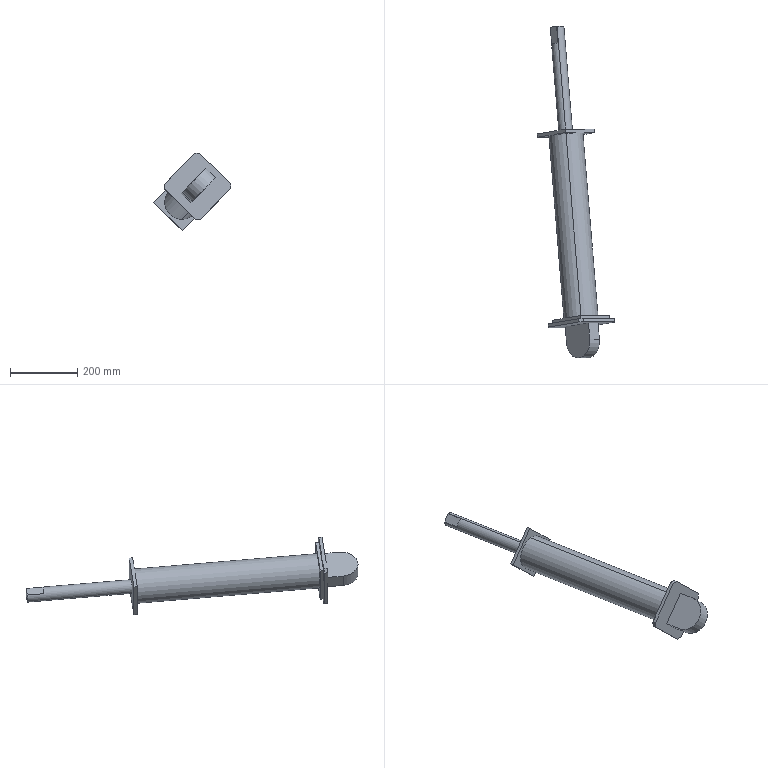Part | SolidWorks | features BaseBody 1 | 1 solid | 35 faces | box 230.771 x 990.893 x 231.743 mm | volume 5798117 mm3 | plane 30 | cylinder 5 | commonest cylinder face diameters 40.723 x2 102.404 x2 100 x1
STEP:
#1=CARTESIAN_POINT('',(-1330.685,834.679,-2427.636));
#2=VERTEX_POINT('',#1);
#3=CARTESIAN_POINT('',(-1330.685,843.27,-2325.593));
#4=VERTEX_POINT('',#3);
#5=CARTESIAN_POINT('',(-1330.685,838.974,-2376.614));
#6=DIRECTION('',(0.08182,-0.9931,0.08361));
#7=DIRECTION('',(0.,-0.08389,-0.9965));
#8=AXIS2_PLACEMENT_3D('',#5,#6,#7);
#9=CIRCLE('',#8,51.202);
#10=EDGE_CURVE('',#2,#4,#9,.T.);
#11=ORIENTED_EDGE('',*,*,#10,.T.);
#12=CARTESIAN_POINT('',(-1285.682,297.046,-2279.609));
#13=VERTEX_POINT('',#12);
#14=CARTESIAN_POINT('',(-1330.685,843.27,-2325.593));
#15=DIRECTION('',(0.08182,-0.9931,0.08361));
#16=VECTOR('',#15,1000.);
#17=LINE('',#14,#16);
#18=EDGE_CURVE('',#4,#13,#17,.T.);
#19=ORIENTED_EDGE('',*,*,#18,.T.);
#20=CARTESIAN_POINT('',(-1285.682,288.456,-2381.652));
#21=VERTEX_POINT('',#20);
#22=CARTESIAN_POINT('',(-1285.682,292.751,-2330.631));
#23=DIRECTION('',(-0.08182,0.9931,-0.08361));
#24=DIRECTION('',(0.,-0.08389,-0.9965));
#25=AXIS2_PLACEMENT_3D('',#22,#23,#24);
#26=CIRCLE('',#25,51.202);
#27=EDGE_CURVE('',#13,#21,#26,.T.);
#28=ORIENTED_EDGE('',*,*,#27,.T.);
#29=CARTESIAN_POINT('',(-1330.685,834.679,-2427.636));
#30=DIRECTION('',(0.08182,-0.9931,0.08361));
#31=VECTOR('',#30,1000.);
#32=LINE('',#29,#31);
#33=EDGE_CURVE('',#2,#21,#32,.T.);
#34=ORIENTED_EDGE('',*,*,#33,.F.);
#35=EDGE_LOOP('',(#11,#19,#28,#34));
#36=FACE_OUTER_BOUND('',#35,.T.);
#37=CARTESIAN_POINT('',(-1330.685,838.974,-2376.614));
#38=DIRECTION('',(0.08182,-0.9931,0.08361));
#39=DIRECTION('',(0.,-0.08389,-0.9965));
#40=AXIS2_PLACEMENT_3D('',#37,#38,#39);
#41=CYLINDRICAL_SURFACE('',#40,51.202);
#42=ADVANCED_FACE('',(#36),#41,.T.);
#43=CARTESIAN_POINT('',(-1336.993,1163.354,-2404.505));
#44=VERTEX_POINT('',#43);
#45=CARTESIAN_POINT('',(-1357.278,1163.451,-2383.497));
#46=VERTEX_POINT('',#45);
#47=CARTESIAN_POINT('',(-1357.278,1161.743,-2403.786));
#48=DIRECTION('',(0.08182,-0.9931,0.08361));
#49=DIRECTION('',(0.,-0.08389,-0.9965));
#50=AXIS2_PLACEMENT_3D('',#47,#48,#49);
#51=CIRCLE('',#50,20.361);
#52=EDGE_CURVE('',#44,#46,#51,.T.);
#53=ORIENTED_EDGE('',*,*,#52,.T.);
#54=CARTESIAN_POINT('',(-1331.503,850.614,-2357.161));
#55=VERTEX_POINT('',#54);
#56=CARTESIAN_POINT('',(-1357.278,1163.451,-2383.497));
#57=DIRECTION('',(0.08182,-0.9931,0.08361));
#58=VECTOR('',#57,1000.);
#59=LINE('',#56,#58);
#60=EDGE_CURVE('',#46,#55,#59,.T.);
#61=ORIENTED_EDGE('',*,*,#60,.T.);
#62=CARTESIAN_POINT('',(-1331.503,847.198,-2397.74));
#63=VERTEX_POINT('',#62);
#64=CARTESIAN_POINT('',(-1331.503,848.906,-2377.45));
#65=DIRECTION('',(0.08182,-0.9931,0.08361));
#66=DIRECTION('',(0.,-0.08389,-0.9965));
#67=AXIS2_PLACEMENT_3D('',#64,#65,#66);
#68=CIRCLE('',#67,20.361);
#69=EDGE_CURVE('',#63,#55,#68,.T.);
#70=ORIENTED_EDGE('',*,*,#69,.F.);
#71=CARTESIAN_POINT('',(-1357.278,1160.035,-2424.076));
#72=VERTEX_POINT('',#71);
#73=CARTESIAN_POINT('',(-1357.278,1160.035,-2424.076));
#74=DIRECTION('',(0.08182,-0.9931,0.08361));
#75=VECTOR('',#74,1000.);
#76=LINE('',#73,#75);
#77=EDGE_CURVE('',#72,#63,#76,.T.);
#78=ORIENTED_EDGE('',*,*,#77,.F.);
#79=CARTESIAN_POINT('',(-1356.122,1160.132,-2424.051));
#80=VERTEX_POINT('',#79);
#81=CARTESIAN_POINT('',(-1357.278,1161.743,-2403.786));
#82=DIRECTION('',(0.08182,-0.9931,0.08361));
#83=DIRECTION('',(0.,-0.08389,-0.9965));
#84=AXIS2_PLACEMENT_3D('',#81,#82,#83);
#85=CIRCLE('',#84,20.361);
#86=EDGE_CURVE('',#72,#80,#85,.T.);
#87=ORIENTED_EDGE('',*,*,#86,.T.);
#88=CARTESIAN_POINT('',(-1352.031,1110.475,-2419.871));
#89=VERTEX_POINT('',#88);
#90=CARTESIAN_POINT('',(-1356.122,1160.132,-2424.051));
#91=DIRECTION('',(0.08182,-0.9931,0.08361));
#92=VECTOR('',#91,1000.);
#93=LINE('',#90,#92);
#94=EDGE_CURVE('',#80,#89,#93,.T.);
#95=ORIENTED_EDGE('',*,*,#94,.T.);
#96=CARTESIAN_POINT('',(-1332.902,1113.697,-2400.325));
#97=VERTEX_POINT('',#96);
#98=CARTESIAN_POINT('',(-1353.186,1112.086,-2399.606));
#99=DIRECTION('',(0.08182,-0.9931,0.08361));
#100=DIRECTION('',(0.,-0.08389,-0.9965));
#101=AXIS2_PLACEMENT_3D('',#98,#99,#100);
#102=CIRCLE('',#101,20.361);
#103=EDGE_CURVE('',#89,#97,#102,.T.);
#104=ORIENTED_EDGE('',*,*,#103,.T.);
#105=CARTESIAN_POINT('',(-1336.993,1163.354,-2404.505));
#106=DIRECTION('',(-0.08182,0.9931,-0.08361));
#107=VECTOR('',#106,1000.);
#108=LINE('',#105,#107);
#109=EDGE_CURVE('',#97,#44,#108,.T.);
#110=ORIENTED_EDGE('',*,*,#109,.T.);
#111=EDGE_LOOP('',(#53,#61,#70,#78,#87,#95,#104,#110));
#112=FACE_OUTER_BOUND('',#111,.T.);
#113=CARTESIAN_POINT('',(-1357.278,1161.743,-2403.786));
#114=DIRECTION('',(0.08182,-0.9931,0.08361));
#115=DIRECTION('',(0.,-0.08389,-0.9965));
#116=AXIS2_PLACEMENT_3D('',#113,#114,#115);
#117=CYLINDRICAL_SURFACE('',#116,20.361);
#118=ADVANCED_FACE('',(#112),#117,.T.);
#119=ORIENTED_EDGE('',*,*,#18,.F.);
#120=CARTESIAN_POINT('',(-1330.685,838.974,-2376.614));
#121=DIRECTION('',(0.08182,-0.9931,0.08361));
#122=DIRECTION('',(0.,-0.08389,-0.9965));
#123=AXIS2_PLACEMENT_3D('',#120,#121,#122);
#124=CIRCLE('',#123,51.202);
#125=EDGE_CURVE('',#4,#2,#124,.T.);
#126=ORIENTED_EDGE('',*,*,#125,.T.);
#127=ORIENTED_EDGE('',*,*,#33,.T.);
#128=CARTESIAN_POINT('',(-1285.682,292.751,-2330.631));
#129=DIRECTION('',(-0.08182,0.9931,-0.08361));
#130=DIRECTION('',(0.,-0.08389,-0.9965));
#131=AXIS2_PLACEMENT_3D('',#128,#129,#130);
#132=CIRCLE('',#131,51.202);
#133=EDGE_CURVE('',#21,#13,#132,.T.);
#134=ORIENTED_EDGE('',*,*,#133,.T.);
#135=EDGE_LOOP('',(#119,#126,#127,#134));
#136=FACE_OUTER_BOUND('',#135,.T.);
#137=CARTESIAN_POINT('',(-1330.685,838.974,-2376.614));
#138=DIRECTION('',(0.08182,-0.9931,0.08361));
#139=DIRECTION('',(0.,-0.08389,-0.9965));
#140=AXIS2_PLACEMENT_3D('',#137,#138,#139);
#141=CYLINDRICAL_SURFACE('',#140,51.202);
#142=ADVANCED_FACE('',(#136),#141,.T.);
#143=ORIENTED_EDGE('',*,*,#10,.F.);
#144=ORIENTED_EDGE('',*,*,#125,.F.);
#145=EDGE_LOOP('',(#143,#144));
#146=FACE_BOUND('',#145,.T.);
#147=CARTESIAN_POINT('',(-1329.482,831.955,-2461.168));
#148=VERTEX_POINT('',#147);
#149=CARTESIAN_POINT('',(-1415.245,831.955,-2377.234));
#150=VERTEX_POINT('',#149);
#151=CARTESIAN_POINT('',(-1329.482,831.955,-2461.168));
#152=DIRECTION('',(-0.7147,0.,0.6994));
#153=VECTOR('',#152,1000.);
#154=LINE('',#151,#153);
#155=EDGE_CURVE('',#148,#150,#154,.T.);
#156=ORIENTED_EDGE('',*,*,#155,.F.);
#157=CARTESIAN_POINT('',(-1246.125,845.993,-2375.994));
#158=VERTEX_POINT('',#157);
#159=CARTESIAN_POINT('',(-1246.125,845.993,-2375.994));
#160=DIRECTION('',(-0.6946,-0.117,-0.7098));
#161=VECTOR('',#160,1000.);
#162=LINE('',#159,#161);
#163=EDGE_CURVE('',#158,#148,#162,.T.);
#164=ORIENTED_EDGE('',*,*,#163,.F.);
#165=CARTESIAN_POINT('',(-1331.888,845.993,-2292.061));
#166=VERTEX_POINT('',#165);
#167=CARTESIAN_POINT('',(-1331.888,845.993,-2292.061));
#168=DIRECTION('',(0.7147,0.,-0.6994));
#169=VECTOR('',#168,1000.);
#170=LINE('',#167,#169);
#171=EDGE_CURVE('',#166,#158,#170,.T.);
#172=ORIENTED_EDGE('',*,*,#171,.F.);
#173=CARTESIAN_POINT('',(-1415.245,831.955,-2377.234));
#174=DIRECTION('',(0.6946,0.117,0.7098));
#175=VECTOR('',#174,1000.);
#176=LINE('',#173,#175);
#177=EDGE_CURVE('',#150,#166,#176,.T.);
#178=ORIENTED_EDGE('',*,*,#177,.F.);
#179=EDGE_LOOP('',(#156,#164,#172,#178));
#180=FACE_OUTER_BOUND('',#179,.T.);
#181=CARTESIAN_POINT('',(-1330.685,838.974,-2376.614));
#182=DIRECTION('',(-0.08182,0.9931,-0.08361));
#183=DIRECTION('',(0.,0.08389,0.9965));
#184=AXIS2_PLACEMENT_3D('',#181,#182,#183);
#185=PLANE('',#184);
#186=ADVANCED_FACE('',(#146,#180),#185,.F.);
#187=ORIENTED_EDGE('',*,*,#133,.F.);
#188=ORIENTED_EDGE('',*,*,#27,.F.);
#189=EDGE_LOOP('',(#187,#188));
#190=FACE_BOUND('',#189,.T.);
#191=CARTESIAN_POINT('',(-1201.122,299.77,-2330.01));
#192=VERTEX_POINT('',#191);
#193=CARTESIAN_POINT('',(-1284.479,285.732,-2415.184));
#194=VERTEX_POINT('',#193);
#195=CARTESIAN_POINT('',(-1201.122,299.77,-2330.01));
#196=DIRECTION('',(-0.6946,-0.117,-0.7098));
#197=VECTOR('',#196,1000.);
#198=LINE('',#195,#197);
#199=EDGE_CURVE('',#192,#194,#198,.T.);
#200=ORIENTED_EDGE('',*,*,#199,.T.);
#201=CARTESIAN_POINT('',(-1370.242,285.732,-2331.251));
#202=VERTEX_POINT('',#201);
#203=CARTESIAN_POINT('',(-1284.479,285.732,-2415.184));
#204=DIRECTION('',(-0.7147,0.,0.6994));
#205=VECTOR('',#204,1000.);
#206=LINE('',#203,#205);
#207=EDGE_CURVE('',#194,#202,#206,.T.);
#208=ORIENTED_EDGE('',*,*,#207,.T.);
#209=CARTESIAN_POINT('',(-1286.885,299.77,-2246.077));
#210=VERTEX_POINT('',#209);
#211=CARTESIAN_POINT('',(-1370.242,285.732,-2331.251));
#212=DIRECTION('',(0.6946,0.117,0.7098));
#213=VECTOR('',#212,1000.);
#214=LINE('',#211,#213);
#215=EDGE_CURVE('',#202,#210,#214,.T.);
#216=ORIENTED_EDGE('',*,*,#215,.T.);
#217=CARTESIAN_POINT('',(-1286.885,299.77,-2246.077));
#218=DIRECTION('',(0.7147,0.,-0.6994));
#219=VECTOR('',#218,1000.);
#220=LINE('',#217,#219);
#221=EDGE_CURVE('',#210,#192,#220,.T.);
#222=ORIENTED_EDGE('',*,*,#221,.T.);
#223=EDGE_LOOP('',(#200,#208,#216,#222));
#224=FACE_OUTER_BOUND('',#223,.T.);
#225=CARTESIAN_POINT('',(-1285.682,292.751,-2330.631));
#226=DIRECTION('',(-0.08182,0.9931,-0.08361));
#227=DIRECTION('',(0.,0.08389,0.9965));
#228=AXIS2_PLACEMENT_3D('',#225,#226,#227);
#229=PLANE('',#228);
#230=ADVANCED_FACE('',(#190,#224),#229,.T.);
#231=CARTESIAN_POINT('',(-1332.706,855.925,-2292.897));
#232=VERTEX_POINT('',#231);
#233=CARTESIAN_POINT('',(-1332.706,855.925,-2292.897));
#234=DIRECTION('',(0.08182,-0.9931,0.08361));
#235=VECTOR('',#234,1000.);
#236=LINE('',#233,#235);
#237=EDGE_CURVE('',#232,#166,#236,.T.);
#238=ORIENTED_EDGE('',*,*,#237,.F.);
#239=CARTESIAN_POINT('',(-1416.063,841.887,-2378.07));
#240=VERTEX_POINT('',#239);
#241=CARTESIAN_POINT('',(-1416.063,841.887,-2378.07));
#242=DIRECTION('',(0.6946,0.117,0.7098));
#243=VECTOR('',#242,1000.);
#244=LINE('',#241,#243);
#245=EDGE_CURVE('',#240,#232,#244,.T.);
#246=ORIENTED_EDGE('',*,*,#245,.F.);
#247=CARTESIAN_POINT('',(-1415.245,831.955,-2377.234));
#248=DIRECTION('',(-0.08182,0.9931,-0.08361));
#249=VECTOR('',#248,1000.);
#250=LINE('',#247,#249);
#251=EDGE_CURVE('',#150,#240,#250,.T.);
#252=ORIENTED_EDGE('',*,*,#251,.F.);
#253=ORIENTED_EDGE('',*,*,#177,.T.);
#254=EDGE_LOOP('',(#238,#246,#252,#253));
#255=FACE_OUTER_BOUND('',#254,.T.);
#256=CARTESIAN_POINT('',(-1416.063,841.887,-2378.07));
#257=DIRECTION('',(0.7147,0.,-0.6994));
#258=DIRECTION('',(-0.6994,0.,-0.7147));
#259=AXIS2_PLACEMENT_3D('',#256,#257,#258);
#260=PLANE('',#259);
#261=ADVANCED_FACE('',(#255),#260,.F.);
#262=ORIENTED_EDGE('',*,*,#251,.T.);
#263=CARTESIAN_POINT('',(-1330.3,841.887,-2462.004));
#264=VERTEX_POINT('',#263);
#265=CARTESIAN_POINT('',(-1416.063,841.887,-2378.07));
#266=DIRECTION('',(-0.7147,0.,0.6994));
#267=VECTOR('',#266,1000.);
#268=LINE('',#265,#267);
#269=EDGE_CURVE('',#264,#240,#268,.T.);
#270=ORIENTED_EDGE('',*,*,#269,.F.);
#271=CARTESIAN_POINT('',(-1330.3,841.887,-2462.004));
#272=DIRECTION('',(-0.08182,0.9931,-0.08361));
#273=VECTOR('',#272,1000.);
#274=LINE('',#271,#273);
#275=EDGE_CURVE('',#148,#264,#274,.T.);
#276=ORIENTED_EDGE('',*,*,#275,.F.);
#277=ORIENTED_EDGE('',*,*,#155,.T.);
#278=EDGE_LOOP('',(#262,#270,#276,#277));
#279=FACE_OUTER_BOUND('',#278,.T.);
#280=CARTESIAN_POINT('',(-1416.063,841.887,-2378.07));
#281=DIRECTION('',(0.6946,0.117,0.7098));
#282=DIRECTION('',(0.7147,0.,-0.6994));
#283=AXIS2_PLACEMENT_3D('',#280,#281,#282);
#284=PLANE('',#283);
#285=ADVANCED_FACE('',(#279),#284,.F.);
#286=ORIENTED_EDGE('',*,*,#275,.T.);
#287=CARTESIAN_POINT('',(-1246.943,855.925,-2376.83));
#288=VERTEX_POINT('',#287);
#289=CARTESIAN_POINT('',(-1246.943,855.925,-2376.83));
#290=DIRECTION('',(-0.6946,-0.117,-0.7098));
#291=VECTOR('',#290,1000.);
#292=LINE('',#289,#291);
#293=EDGE_CURVE('',#288,#264,#292,.T.);
#294=ORIENTED_EDGE('',*,*,#293,.F.);
#295=CARTESIAN_POINT('',(-1246.125,845.993,-2375.994));
#296=DIRECTION('',(-0.08182,0.9931,-0.08361));
#297=VECTOR('',#296,1000.);
#298=LINE('',#295,#297);
#299=EDGE_CURVE('',#158,#288,#298,.T.);
#300=ORIENTED_EDGE('',*,*,#299,.F.);
#301=ORIENTED_EDGE('',*,*,#163,.T.);
#302=EDGE_LOOP('',(#286,#294,#300,#301));
#303=FACE_OUTER_BOUND('',#302,.T.);
#304=CARTESIAN_POINT('',(-1330.3,841.887,-2462.004));
#305=DIRECTION('',(-0.7147,0.,0.6994));
#306=DIRECTION('',(0.6994,0.,0.7147));
#307=AXIS2_PLACEMENT_3D('',#304,#305,#306);
#308=PLANE('',#307);
#309=ADVANCED_FACE('',(#303),#308,.F.);
#310=ORIENTED_EDGE('',*,*,#299,.T.);
#311=CARTESIAN_POINT('',(-1332.706,855.925,-2292.897));
#312=DIRECTION('',(0.7147,0.,-0.6994));
#313=VECTOR('',#312,1000.);
#314=LINE('',#311,#313);
#315=EDGE_CURVE('',#232,#288,#314,.T.);
#316=ORIENTED_EDGE('',*,*,#315,.F.);
#317=ORIENTED_EDGE('',*,*,#237,.T.);
#318=ORIENTED_EDGE('',*,*,#171,.T.);
#319=EDGE_LOOP('',(#310,#316,#317,#318));
#320=FACE_OUTER_BOUND('',#319,.T.);
#321=CARTESIAN_POINT('',(-1332.706,855.925,-2292.897));
#322=DIRECTION('',(-0.6946,-0.117,-0.7098));
#323=DIRECTION('',(-0.7147,0.,0.6994));
#324=AXIS2_PLACEMENT_3D('',#321,#322,#323);
#325=PLANE('',#324);
#326=ADVANCED_FACE('',(#320),#325,.F.);
#327=CARTESIAN_POINT('',(-1369.424,275.8,-2330.415));
#328=VERTEX_POINT('',#327);
#329=CARTESIAN_POINT('',(-1370.242,285.732,-2331.251));
#330=DIRECTION('',(0.08182,-0.9931,0.08361));
#331=VECTOR('',#330,1000.);
#332=LINE('',#329,#331);
#333=EDGE_CURVE('',#202,#328,#332,.T.);
#334=ORIENTED_EDGE('',*,*,#333,.F.);
#335=ORIENTED_EDGE('',*,*,#207,.F.);
#336=CARTESIAN_POINT('',(-1283.661,275.8,-2414.348));
#337=VERTEX_POINT('',#336);
#338=CARTESIAN_POINT('',(-1284.479,285.732,-2415.184));
#339=DIRECTION('',(-0.08182,0.9931,-0.08361));
#340=VECTOR('',#339,1000.);
#341=LINE('',#338,#340);
#342=EDGE_CURVE('',#337,#194,#341,.T.);
#343=ORIENTED_EDGE('',*,*,#342,.F.);
#344=CARTESIAN_POINT('',(-1369.424,275.8,-2330.415));
#345=DIRECTION('',(0.7147,0.,-0.6994));
#346=VECTOR('',#345,1000.);
#347=LINE('',#344,#346);
#348=EDGE_CURVE('',#328,#337,#347,.T.);
#349=ORIENTED_EDGE('',*,*,#348,.F.);
#350=EDGE_LOOP('',(#334,#335,#343,#349));
#351=FACE_OUTER_BOUND('',#350,.T.);
#352=CARTESIAN_POINT('',(-1370.242,285.732,-2331.251));
#353=DIRECTION('',(0.6946,0.117,0.7098));
#354=DIRECTION('',(0.7147,0.,-0.6994));
#355=AXIS2_PLACEMENT_3D('',#352,#353,#354);
#356=PLANE('',#355);
#357=ADVANCED_FACE('',(#351),#356,.F.);
#358=ORIENTED_EDGE('',*,*,#342,.T.);
#359=ORIENTED_EDGE('',*,*,#199,.F.);
#360=CARTESIAN_POINT('',(-1200.304,289.838,-2329.174));
#361=VERTEX_POINT('',#360);
#362=CARTESIAN_POINT('',(-1200.304,289.838,-2329.174));
#363=DIRECTION('',(-0.08182,0.9931,-0.08361));
#364=VECTOR('',#363,1000.);
#365=LINE('',#362,#364);
#366=EDGE_CURVE('',#361,#192,#365,.T.);
#367=ORIENTED_EDGE('',*,*,#366,.F.);
#368=CARTESIAN_POINT('',(-1283.661,275.8,-2414.348));
#369=DIRECTION('',(0.6946,0.117,0.7098));
#370=VECTOR('',#369,1000.);
#371=LINE('',#368,#370);
#372=EDGE_CURVE('',#337,#361,#371,.T.);
#373=ORIENTED_EDGE('',*,*,#372,.F.);
#374=EDGE_LOOP('',(#358,#359,#367,#373));
#375=FACE_OUTER_BOUND('',#374,.T.);
#376=CARTESIAN_POINT('',(-1284.479,285.732,-2415.184));
#377=DIRECTION('',(-0.7147,0.,0.6994));
#378=DIRECTION('',(0.6994,0.,0.7147));
#379=AXIS2_PLACEMENT_3D('',#376,#377,#378);
#380=PLANE('',#379);
#381=ADVANCED_FACE('',(#375),#380,.F.);
#382=ORIENTED_EDGE('',*,*,#366,.T.);
#383=ORIENTED_EDGE('',*,*,#221,.F.);
#384=CARTESIAN_POINT('',(-1286.067,289.838,-2245.241));
#385=VERTEX_POINT('',#384);
#386=CARTESIAN_POINT('',(-1286.885,299.77,-2246.077));
#387=DIRECTION('',(-0.08182,0.9931,-0.08361));
#388=VECTOR('',#387,1000.);
#389=LINE('',#386,#388);
#390=EDGE_CURVE('',#385,#210,#389,.T.);
#391=ORIENTED_EDGE('',*,*,#390,.F.);
#392=CARTESIAN_POINT('',(-1286.067,289.838,-2245.241));
#393=DIRECTION('',(-0.7147,0.,0.6994));
#394=VECTOR('',#393,1000.);
#395=LINE('',#392,#394);
#396=EDGE_CURVE('',#361,#385,#395,.T.);
#397=ORIENTED_EDGE('',*,*,#396,.F.);
#398=EDGE_LOOP('',(#382,#383,#391,#397));
#399=FACE_OUTER_BOUND('',#398,.T.);
#400=CARTESIAN_POINT('',(-1286.885,299.77,-2246.077));
#401=DIRECTION('',(-0.6946,-0.117,-0.7098));
#402=DIRECTION('',(-0.7147,0.,0.6994));
#403=AXIS2_PLACEMENT_3D('',#400,#401,#402);
#404=PLANE('',#403);
#405=ADVANCED_FACE('',(#399),#404,.F.);
#406=ORIENTED_EDGE('',*,*,#390,.T.);
#407=ORIENTED_EDGE('',*,*,#215,.F.);
#408=ORIENTED_EDGE('',*,*,#333,.T.);
#409=CARTESIAN_POINT('',(-1286.067,289.838,-2245.241));
#410=DIRECTION('',(-0.6946,-0.117,-0.7098));
#411=VECTOR('',#410,1000.);
#412=LINE('',#409,#411);
#413=EDGE_CURVE('',#385,#328,#412,.T.);
#414=ORIENTED_EDGE('',*,*,#413,.F.);
#415=EDGE_LOOP('',(#406,#407,#408,#414));
#416=FACE_OUTER_BOUND('',#415,.T.);
#417=CARTESIAN_POINT('',(-1370.242,285.732,-2331.251));
#418=DIRECTION('',(0.7147,0.,-0.6994));
#419=DIRECTION('',(-0.6994,0.,-0.7147));
#420=AXIS2_PLACEMENT_3D('',#417,#418,#419);
#421=PLANE('',#420);
#422=ADVANCED_FACE('',(#416),#421,.F.);
#423=ORIENTED_EDGE('',*,*,#69,.T.);
#424=CARTESIAN_POINT('',(-1331.503,848.906,-2377.45));
#425=DIRECTION('',(0.08182,-0.9931,0.08361));
#426=DIRECTION('',(0.,-0.08389,-0.9965));
#427=AXIS2_PLACEMENT_3D('',#424,#425,#426);
#428=CIRCLE('',#427,20.361);
#429=EDGE_CURVE('',#55,#63,#428,.T.);
#430=ORIENTED_EDGE('',*,*,#429,.T.);
#431=EDGE_LOOP('',(#423,#430));
#432=FACE_BOUND('',#431,.T.);
#433=ORIENTED_EDGE('',*,*,#293,.T.);
#434=ORIENTED_EDGE('',*,*,#269,.T.);
#435=ORIENTED_EDGE('',*,*,#245,.T.);
#436=ORIENTED_EDGE('',*,*,#315,.T.);
#437=EDGE_LOOP('',(#433,#434,#435,#436));
#438=FACE_OUTER_BOUND('',#437,.T.);
#439=CARTESIAN_POINT('',(-1331.503,848.906,-2377.45));
#440=DIRECTION('',(-0.08182,0.9931,-0.08361));
#441=DIRECTION('',(0.,0.08389,0.9965));
#442=AXIS2_PLACEMENT_3D('',#439,#440,#441);
#443=PLANE('',#442);
#444=ADVANCED_FACE('',(#432,#438),#443,.T.);
#445=ORIENTED_EDGE('',*,*,#348,.T.);
#446=ORIENTED_EDGE('',*,*,#372,.T.);
#447=ORIENTED_EDGE('',*,*,#396,.T.);
#448=ORIENTED_EDGE('',*,*,#413,.T.);
#449=EDGE_LOOP('',(#445,#446,#447,#448));
#450=FACE_BOUND('',#449,.T.);
#451=CARTESIAN_POINT('',(-1279.22,291.593,-2231.097));
#452=VERTEX_POINT('',#451);
#453=CARTESIAN_POINT('',(-1186.311,291.593,-2322.025));
#454=VERTEX_POINT('',#453);
#455=CARTESIAN_POINT('',(-1279.22,291.593,-2231.097));
#456=DIRECTION('',(0.7147,0.,-0.6994));
#457=VECTOR('',#456,1000.);
#458=LINE('',#455,#457);
#459=EDGE_CURVE('',#452,#454,#458,.T.);
#460=ORIENTED_EDGE('',*,*,#459,.T.);
#461=CARTESIAN_POINT('',(-1186.111,290.423,-2336.117));
#462=VERTEX_POINT('',#461);
#463=CARTESIAN_POINT('',(-1186.311,291.593,-2322.025));
#464=DIRECTION('',(0.01417,-0.08272,-0.9965));
#465=VECTOR('',#464,1000.);
#466=LINE('',#463,#465);
#467=EDGE_CURVE('',#454,#462,#466,.T.);
#468=ORIENTED_EDGE('',*,*,#467,.T.);
#469=CARTESIAN_POINT('',(-1276.414,275.216,-2428.388));
#470=VERTEX_POINT('',#469);
#471=CARTESIAN_POINT('',(-1186.111,290.423,-2336.117));
#472=DIRECTION('',(-0.6946,-0.117,-0.7098));
#473=VECTOR('',#472,1000.);
#474=LINE('',#471,#473);
#475=EDGE_CURVE('',#462,#470,#474,.T.);
#476=ORIENTED_EDGE('',*,*,#475,.T.);
#477=CARTESIAN_POINT('',(-1290.507,274.046,-2428.492));
#478=VERTEX_POINT('',#477);
#479=CARTESIAN_POINT('',(-1276.414,275.216,-2428.388));
#480=DIRECTION('',(-0.9965,-0.08272,-0.007309));
#481=VECTOR('',#480,1000.);
#482=LINE('',#479,#481);
#483=EDGE_CURVE('',#470,#478,#482,.T.);
#484=ORIENTED_EDGE('',*,*,#483,.T.);
#485=CARTESIAN_POINT('',(-1383.417,274.046,-2337.564));
#486=VERTEX_POINT('',#485);
#487=CARTESIAN_POINT('',(-1290.507,274.046,-2428.492));
#488=DIRECTION('',(-0.7147,0.,0.6994));
#489=VECTOR('',#488,1000.);
#490=LINE('',#487,#489);
#491=EDGE_CURVE('',#478,#486,#490,.T.);
#492=ORIENTED_EDGE('',*,*,#491,.T.);
#493=CARTESIAN_POINT('',(-1383.617,275.216,-2323.472));
#494=VERTEX_POINT('',#493);
#495=CARTESIAN_POINT('',(-1383.417,274.046,-2337.564));
#496=DIRECTION('',(-0.01417,0.08272,0.9965));
#497=VECTOR('',#496,1000.);
#498=LINE('',#495,#497);
#499=EDGE_CURVE('',#486,#494,#498,.T.);
#500=ORIENTED_EDGE('',*,*,#499,.T.);
#501=CARTESIAN_POINT('',(-1293.314,290.423,-2231.2));
#502=VERTEX_POINT('',#501);
#503=CARTESIAN_POINT('',(-1383.617,275.216,-2323.472));
#504=DIRECTION('',(0.6946,0.117,0.7098));
#505=VECTOR('',#504,1000.);
#506=LINE('',#503,#505);
#507=EDGE_CURVE('',#494,#502,#506,.T.);
#508=ORIENTED_EDGE('',*,*,#507,.T.);
#509=CARTESIAN_POINT('',(-1293.314,290.423,-2231.2));
#510=DIRECTION('',(0.9965,0.08272,0.007309));
#511=VECTOR('',#510,1000.);
#512=LINE('',#509,#511);
#513=EDGE_CURVE('',#502,#452,#512,.T.);
#514=ORIENTED_EDGE('',*,*,#513,.T.);
#515=EDGE_LOOP('',(#460,#468,#476,#484,#492,#500,#508,#514));
#516=FACE_OUTER_BOUND('',#515,.T.);
#517=CARTESIAN_POINT('',(-1284.864,282.819,-2329.794));
#518=DIRECTION('',(-0.08182,0.9931,-0.08361));
#519=DIRECTION('',(0.,0.08389,0.9965));
#520=AXIS2_PLACEMENT_3D('',#517,#518,#519);
#521=PLANE('',#520);
#522=ADVANCED_FACE('',(#450,#516),#521,.T.);
#523=ORIENTED_EDGE('',*,*,#60,.F.);
#524=CARTESIAN_POINT('',(-1358.433,1163.354,-2383.522));
#525=VERTEX_POINT('',#524);
#526=CARTESIAN_POINT('',(-1357.278,1161.743,-2403.786));
#527=DIRECTION('',(0.08182,-0.9931,0.08361));
#528=DIRECTION('',(0.,-0.08389,-0.9965));
#529=AXIS2_PLACEMENT_3D('',#526,#527,#528);
#530=CIRCLE('',#529,20.361);
#531=EDGE_CURVE('',#46,#525,#530,.T.);
#532=ORIENTED_EDGE('',*,*,#531,.T.);
#533=CARTESIAN_POINT('',(-1354.342,1113.697,-2379.341));
#534=VERTEX_POINT('',#533);
#535=CARTESIAN_POINT('',(-1358.433,1163.354,-2383.522));
#536=DIRECTION('',(0.08182,-0.9931,0.08361));
#537=VECTOR('',#536,1000.);
#538=LINE('',#535,#537);
#539=EDGE_CURVE('',#525,#534,#538,.T.);
#540=ORIENTED_EDGE('',*,*,#539,.T.);
#541=CARTESIAN_POINT('',(-1373.471,1110.475,-2398.887));
#542=VERTEX_POINT('',#541);
#543=CARTESIAN_POINT('',(-1353.186,1112.086,-2399.606));
#544=DIRECTION('',(0.08182,-0.9931,0.08361));
#545=DIRECTION('',(0.,-0.08389,-0.9965));
#546=AXIS2_PLACEMENT_3D('',#543,#544,#545);
#547=CIRCLE('',#546,20.361);
#548=EDGE_CURVE('',#534,#542,#547,.T.);
#549=ORIENTED_EDGE('',*,*,#548,.T.);
#550=CARTESIAN_POINT('',(-1377.562,1160.132,-2403.068));
#551=VERTEX_POINT('',#550);
#552=CARTESIAN_POINT('',(-1377.562,1160.132,-2403.068));
#553=DIRECTION('',(-0.08182,0.9931,-0.08361));
#554=VECTOR('',#553,1000.);
#555=LINE('',#552,#554);
#556=EDGE_CURVE('',#542,#551,#555,.T.);
#557=ORIENTED_EDGE('',*,*,#556,.T.);
#558=CARTESIAN_POINT('',(-1357.278,1161.743,-2403.786));
#559=DIRECTION('',(0.08182,-0.9931,0.08361));
#560=DIRECTION('',(0.,-0.08389,-0.9965));
#561=AXIS2_PLACEMENT_3D('',#558,#559,#560);
#562=CIRCLE('',#561,20.361);
#563=EDGE_CURVE('',#551,#72,#562,.T.);
#564=ORIENTED_EDGE('',*,*,#563,.T.);
#565=ORIENTED_EDGE('',*,*,#77,.T.);
#566=ORIENTED_EDGE('',*,*,#429,.F.);
#567=EDGE_LOOP('',(#523,#532,#540,#549,#557,#564,#565,#566));
#568=FACE_OUTER_BOUND('',#567,.T.);
#569=CARTESIAN_POINT('',(-1357.278,1161.743,-2403.786));
#570=DIRECTION('',(0.08182,-0.9931,0.08361));
#571=DIRECTION('',(0.,-0.08389,-0.9965));
#572=AXIS2_PLACEMENT_3D('',#569,#570,#571);
#573=CYLINDRICAL_SURFACE('',#572,20.361);
#574=ADVANCED_FACE('',(#568),#573,.T.);
#575=CARTESIAN_POINT('',(-1185.493,281.662,-2321.189));
#576=VERTEX_POINT('',#575);
#577=CARTESIAN_POINT('',(-1185.493,281.662,-2321.189));
#578=DIRECTION('',(-0.08182,0.9931,-0.08361));
#579=VECTOR('',#578,1000.);
#580=LINE('',#577,#579);
#581=EDGE_CURVE('',#576,#454,#580,.T.);
#582=ORIENTED_EDGE('',*,*,#581,.F.);
#583=CARTESIAN_POINT('',(-1185.292,280.492,-2335.281));
#584=VERTEX_POINT('',#583);
#585=CARTESIAN_POINT('',(-1185.292,280.492,-2335.281));
#586=DIRECTION('',(-0.01417,0.08272,0.9965));
#587=VECTOR('',#586,1000.);
#588=LINE('',#585,#587);
#589=EDGE_CURVE('',#584,#576,#588,.T.);
#590=ORIENTED_EDGE('',*,*,#589,.F.);
#591=CARTESIAN_POINT('',(-1186.111,290.423,-2336.117));
#592=DIRECTION('',(0.08182,-0.9931,0.08361));
#593=VECTOR('',#592,1000.);
#594=LINE('',#591,#593);
#595=EDGE_CURVE('',#462,#584,#594,.T.);
#596=ORIENTED_EDGE('',*,*,#595,.F.);
#597=ORIENTED_EDGE('',*,*,#467,.F.);
#598=EDGE_LOOP('',(#582,#590,#596,#597));
#599=FACE_OUTER_BOUND('',#598,.T.);
#600=CARTESIAN_POINT('',(-1186.111,290.423,-2336.117));
#601=DIRECTION('',(-0.9965,-0.08272,-0.007309));
#602=DIRECTION('',(0.08272,-0.9966,0.));
#603=AXIS2_PLACEMENT_3D('',#600,#601,#602);
#604=PLANE('',#603);
#605=ADVANCED_FACE('',(#599),#604,.F.);
#606=ORIENTED_EDGE('',*,*,#581,.T.);
#607=ORIENTED_EDGE('',*,*,#459,.F.);
#608=CARTESIAN_POINT('',(-1278.402,281.662,-2230.261));
#609=VERTEX_POINT('',#608);
#610=CARTESIAN_POINT('',(-1279.22,291.593,-2231.097));
#611=DIRECTION('',(-0.08182,0.9931,-0.08361));
#612=VECTOR('',#611,1000.);
#613=LINE('',#610,#612);
#614=EDGE_CURVE('',#609,#452,#613,.T.);
#615=ORIENTED_EDGE('',*,*,#614,.F.);
#616=CARTESIAN_POINT('',(-1285.549,281.662,-2223.267));
#617=DIRECTION('',(-0.7147,0.,0.6994));
#618=VECTOR('',#617,1000.);
#619=LINE('',#616,#618);
#620=EDGE_CURVE('',#576,#609,#619,.T.);
#621=ORIENTED_EDGE('',*,*,#620,.F.);
#622=EDGE_LOOP('',(#606,#607,#615,#621));
#623=FACE_OUTER_BOUND('',#622,.T.);
#624=CARTESIAN_POINT('',(-1286.367,291.593,-2224.103));
#625=DIRECTION('',(-0.6946,-0.117,-0.7098));
#626=DIRECTION('',(-0.7147,0.,0.6994));
#627=AXIS2_PLACEMENT_3D('',#624,#625,#626);
#628=PLANE('',#627);
#629=ADVANCED_FACE('',(#623),#628,.F.);
#630=CARTESIAN_POINT('',(-1292.495,280.492,-2230.364));
#631=VERTEX_POINT('',#630);
#632=CARTESIAN_POINT('',(-1292.495,280.492,-2230.364));
#633=DIRECTION('',(-0.08182,0.9931,-0.08361));
#634=VECTOR('',#633,1000.);
#635=LINE('',#632,#634);
#636=EDGE_CURVE('',#631,#502,#635,.T.);
#637=ORIENTED_EDGE('',*,*,#636,.F.);
#638=CARTESIAN_POINT('',(-1278.402,281.662,-2230.261));
#639=DIRECTION('',(-0.9965,-0.08272,-0.007309));
#640=VECTOR('',#639,1000.);
#641=LINE('',#638,#640);
#642=EDGE_CURVE('',#609,#631,#641,.T.);
#643=ORIENTED_EDGE('',*,*,#642,.F.);
#644=ORIENTED_EDGE('',*,*,#614,.T.);
#645=ORIENTED_EDGE('',*,*,#513,.F.);
#646=EDGE_LOOP('',(#637,#643,#644,#645));
#647=FACE_OUTER_BOUND('',#646,.T.);
#648=CARTESIAN_POINT('',(-1279.22,291.593,-2231.097));
#649=DIRECTION('',(0.01417,-0.08272,-0.9965));
#650=DIRECTION('',(0.,0.9966,-0.08273));
#651=AXIS2_PLACEMENT_3D('',#648,#649,#650);
#652=PLANE('',#651);
#653=ADVANCED_FACE('',(#647),#652,.F.);
#654=ORIENTED_EDGE('',*,*,#636,.T.);
#655=ORIENTED_EDGE('',*,*,#507,.F.);
#656=CARTESIAN_POINT('',(-1382.799,265.284,-2322.636));
#657=VERTEX_POINT('',#656);
#658=CARTESIAN_POINT('',(-1382.799,265.284,-2322.636));
#659=DIRECTION('',(-0.08182,0.9931,-0.08361));
#660=VECTOR('',#659,1000.);
#661=LINE('',#658,#660);
#662=EDGE_CURVE('',#657,#494,#661,.T.);
#663=ORIENTED_EDGE('',*,*,#662,.F.);
#664=CARTESIAN_POINT('',(-1292.495,280.492,-2230.364));
#665=DIRECTION('',(-0.6946,-0.117,-0.7098));
#666=VECTOR('',#665,1000.);
#667=LINE('',#664,#666);
#668=EDGE_CURVE('',#631,#657,#667,.T.);
#669=ORIENTED_EDGE('',*,*,#668,.F.);
#670=EDGE_LOOP('',(#654,#655,#663,#669));
#671=FACE_OUTER_BOUND('',#670,.T.);
#672=CARTESIAN_POINT('',(-1390.564,274.046,-2330.57));
#673=DIRECTION('',(0.7147,0.,-0.6994));
#674=DIRECTION('',(-0.6994,0.,-0.7147));
#675=AXIS2_PLACEMENT_3D('',#672,#673,#674);
#676=PLANE('',#675);
#677=ADVANCED_FACE('',(#671),#676,.F.);
#678=CARTESIAN_POINT('',(-1382.598,264.114,-2336.728));
#679=VERTEX_POINT('',#678);
#680=CARTESIAN_POINT('',(-1382.598,264.114,-2336.728));
#681=DIRECTION('',(-0.08182,0.9931,-0.08361));
#682=VECTOR('',#681,1000.);
#683=LINE('',#680,#682);
#684=EDGE_CURVE('',#679,#486,#683,.T.);
#685=ORIENTED_EDGE('',*,*,#684,.F.);
#686=CARTESIAN_POINT('',(-1382.799,265.284,-2322.636));
#687=DIRECTION('',(0.01417,-0.08272,-0.9965));
#688=VECTOR('',#687,1000.);
#689=LINE('',#686,#688);
#690=EDGE_CURVE('',#657,#679,#689,.T.);
#691=ORIENTED_EDGE('',*,*,#690,.F.);
#692=ORIENTED_EDGE('',*,*,#662,.T.);
#693=ORIENTED_EDGE('',*,*,#499,.F.);
#694=EDGE_LOOP('',(#685,#691,#692,#693));
#695=FACE_OUTER_BOUND('',#694,.T.);
#696=CARTESIAN_POINT('',(-1383.617,275.216,-2323.472));
#697=DIRECTION('',(0.9965,0.08272,0.007309));
#698=DIRECTION('',(-0.08272,0.9966,0.));
#699=AXIS2_PLACEMENT_3D('',#696,#697,#698);
#700=PLANE('',#699);
#701=ADVANCED_FACE('',(#695),#700,.F.);
#702=CARTESIAN_POINT('',(-1289.689,264.114,-2427.656));
#703=VERTEX_POINT('',#702);
#704=CARTESIAN_POINT('',(-1290.507,274.046,-2428.492));
#705=DIRECTION('',(-0.08182,0.9931,-0.08361));
#706=VECTOR('',#705,1000.);
#707=LINE('',#704,#706);
#708=EDGE_CURVE('',#703,#478,#707,.T.);
#709=ORIENTED_EDGE('',*,*,#708,.F.);
#710=CARTESIAN_POINT('',(-1389.745,264.114,-2329.734));
#711=DIRECTION('',(0.7147,0.,-0.6994));
#712=VECTOR('',#711,1000.);
#713=LINE('',#710,#712);
#714=EDGE_CURVE('',#679,#703,#713,.T.);
#715=ORIENTED_EDGE('',*,*,#714,.F.);
#716=ORIENTED_EDGE('',*,*,#684,.T.);
#717=ORIENTED_EDGE('',*,*,#491,.F.);
#718=EDGE_LOOP('',(#709,#715,#716,#717));
#719=FACE_OUTER_BOUND('',#718,.T.);
#720=CARTESIAN_POINT('',(-1390.564,274.046,-2330.57));
#721=DIRECTION('',(0.6946,0.117,0.7098));
#722=DIRECTION('',(0.7147,0.,-0.6994));
#723=AXIS2_PLACEMENT_3D('',#720,#721,#722);
#724=PLANE('',#723);
#725=ADVANCED_FACE('',(#719),#724,.F.);
#726=CARTESIAN_POINT('',(-1275.596,265.284,-2427.552));
#727=VERTEX_POINT('',#726);
#728=CARTESIAN_POINT('',(-1275.596,265.284,-2427.552));
#729=DIRECTION('',(-0.08182,0.9931,-0.08361));
#730=VECTOR('',#729,1000.);
#731=LINE('',#728,#730);
#732=EDGE_CURVE('',#727,#470,#731,.T.);
#733=ORIENTED_EDGE('',*,*,#732,.F.);
#734=CARTESIAN_POINT('',(-1289.689,264.114,-2427.656));
#735=DIRECTION('',(0.9965,0.08272,0.007309));
#736=VECTOR('',#735,1000.);
#737=LINE('',#734,#736);
#738=EDGE_CURVE('',#703,#727,#737,.T.);
#739=ORIENTED_EDGE('',*,*,#738,.F.);
#740=ORIENTED_EDGE('',*,*,#708,.T.);
#741=ORIENTED_EDGE('',*,*,#483,.F.);
#742=EDGE_LOOP('',(#733,#739,#740,#741));
#743=FACE_OUTER_BOUND('',#742,.T.);
#744=CARTESIAN_POINT('',(-1290.507,274.046,-2428.492));
#745=DIRECTION('',(-0.01417,0.08272,0.9965));
#746=DIRECTION('',(0.,-0.9966,0.08273));
#747=AXIS2_PLACEMENT_3D('',#744,#745,#746);
#748=PLANE('',#747);
#749=ADVANCED_FACE('',(#743),#748,.F.);
#750=ORIENTED_EDGE('',*,*,#732,.T.);
#751=ORIENTED_EDGE('',*,*,#475,.F.);
#752=ORIENTED_EDGE('',*,*,#595,.T.);
#753=CARTESIAN_POINT('',(-1275.596,265.284,-2427.552));
#754=DIRECTION('',(0.6946,0.117,0.7098));
#755=VECTOR('',#754,1000.);
#756=LINE('',#753,#755);
#757=EDGE_CURVE('',#727,#584,#756,.T.);
#758=ORIENTED_EDGE('',*,*,#757,.F.);
#759=EDGE_LOOP('',(#750,#751,#752,#758));
#760=FACE_OUTER_BOUND('',#759,.T.);
#761=CARTESIAN_POINT('',(-1283.36,274.046,-2435.486));
#762=DIRECTION('',(-0.7147,0.,0.6994));
#763=DIRECTION('',(0.6994,0.,0.7147));
#764=AXIS2_PLACEMENT_3D('',#761,#762,#763);
#765=PLANE('',#764);
#766=ADVANCED_FACE('',(#760),#765,.F.);
#767=CARTESIAN_POINT('',(-1377.562,1160.132,-2403.068));
#768=DIRECTION('',(0.6946,0.117,0.7098));
#769=VECTOR('',#768,1000.);
#770=LINE('',#767,#769);
#771=EDGE_CURVE('',#551,#525,#770,.T.);
#772=ORIENTED_EDGE('',*,*,#771,.T.);
#773=ORIENTED_EDGE('',*,*,#531,.F.);
#774=ORIENTED_EDGE('',*,*,#52,.F.);
#775=CARTESIAN_POINT('',(-1336.993,1163.354,-2404.505));
#776=DIRECTION('',(-0.6946,-0.117,-0.7098));
#777=VECTOR('',#776,1000.);
#778=LINE('',#775,#777);
#779=EDGE_CURVE('',#44,#80,#778,.T.);
#780=ORIENTED_EDGE('',*,*,#779,.T.);
#781=ORIENTED_EDGE('',*,*,#86,.F.);
#782=ORIENTED_EDGE('',*,*,#563,.F.);
#783=EDGE_LOOP('',(#772,#773,#774,#780,#781,#782));
#784=FACE_OUTER_BOUND('',#783,.T.);
#785=CARTESIAN_POINT('',(-1357.278,1161.743,-2403.786));
#786=DIRECTION('',(-0.08182,0.9931,-0.08361));
#787=DIRECTION('',(0.,0.08389,0.9965));
#788=AXIS2_PLACEMENT_3D('',#785,#786,#787);
#789=PLANE('',#788);
#790=ADVANCED_FACE('',(#784),#789,.T.);
#791=ORIENTED_EDGE('',*,*,#109,.F.);
#792=CARTESIAN_POINT('',(-1352.031,1110.475,-2419.871));
#793=DIRECTION('',(0.6946,0.117,0.7098));
#794=VECTOR('',#793,1000.);
#795=LINE('',#792,#794);
#796=EDGE_CURVE('',#89,#97,#795,.T.);
#797=ORIENTED_EDGE('',*,*,#796,.F.);
#798=ORIENTED_EDGE('',*,*,#94,.F.);
#799=ORIENTED_EDGE('',*,*,#779,.F.);
#800=EDGE_LOOP('',(#791,#797,#798,#799));
#801=FACE_OUTER_BOUND('',#800,.T.);
#802=CARTESIAN_POINT('',(-1277.093,1173.441,-2343.3));
#803=DIRECTION('',(-0.7147,0.,0.6994));
#804=DIRECTION('',(0.6994,0.,0.7147));
#805=AXIS2_PLACEMENT_3D('',#802,#803,#804);
#806=PLANE('',#805);
#807=ADVANCED_FACE('',(#801),#806,.F.);
#808=ORIENTED_EDGE('',*,*,#103,.F.);
#809=ORIENTED_EDGE('',*,*,#796,.T.);
#810=EDGE_LOOP('',(#808,#809));
#811=FACE_OUTER_BOUND('',#810,.T.);
#812=CARTESIAN_POINT('',(-1269.17,1123.785,-2342.87));
#813=DIRECTION('',(0.08182,-0.9931,0.08361));
#814=DIRECTION('',(0.,-0.08389,-0.9965));
#815=AXIS2_PLACEMENT_3D('',#812,#813,#814);
#816=PLANE('',#815);
#817=ADVANCED_FACE('',(#811),#816,.F.);
#818=ORIENTED_EDGE('',*,*,#556,.F.);
#819=CARTESIAN_POINT('',(-1354.342,1113.697,-2379.341));
#820=DIRECTION('',(-0.6946,-0.117,-0.7098));
#821=VECTOR('',#820,1000.);
#822=LINE('',#819,#821);
#823=EDGE_CURVE('',#534,#542,#822,.T.);
#824=ORIENTED_EDGE('',*,*,#823,.F.);
#825=ORIENTED_EDGE('',*,*,#539,.F.);
#826=ORIENTED_EDGE('',*,*,#771,.F.);
#827=EDGE_LOOP('',(#818,#824,#825,#826));
#828=FACE_OUTER_BOUND('',#827,.T.);
#829=CARTESIAN_POINT('',(-1298.534,1173.441,-2322.317));
#830=DIRECTION('',(0.7147,0.,-0.6994));
#831=DIRECTION('',(-0.6994,0.,-0.7147));
#832=AXIS2_PLACEMENT_3D('',#829,#830,#831);
#833=PLANE('',#832);
#834=ADVANCED_FACE('',(#828),#833,.F.);
#835=ORIENTED_EDGE('',*,*,#823,.T.);
#836=ORIENTED_EDGE('',*,*,#548,.F.);
#837=EDGE_LOOP('',(#835,#836));
#838=FACE_OUTER_BOUND('',#837,.T.);
#839=CARTESIAN_POINT('',(-1298.274,1123.785,-2314.386));
#840=DIRECTION('',(0.08182,-0.9931,0.08361));
#841=DIRECTION('',(0.,-0.08389,-0.9965));
#842=AXIS2_PLACEMENT_3D('',#839,#840,#841);
#843=PLANE('',#842);
#844=ADVANCED_FACE('',(#838),#843,.F.);
#845=CARTESIAN_POINT('',(-1263.607,278.737,-2279.481));
#846=VERTEX_POINT('',#845);
#847=CARTESIAN_POINT('',(-1333.071,267.039,-2350.459));
#848=VERTEX_POINT('',#847);
#849=CARTESIAN_POINT('',(-1263.607,278.737,-2279.481));
#850=DIRECTION('',(-0.6946,-0.117,-0.7098));
#851=VECTOR('',#850,1000.);
#852=LINE('',#849,#851);
#853=EDGE_CURVE('',#846,#848,#852,.T.);
#854=ORIENTED_EDGE('',*,*,#853,.F.);
#855=CARTESIAN_POINT('',(-1235.02,278.737,-2307.458));
#856=VERTEX_POINT('',#855);
#857=CARTESIAN_POINT('',(-1235.02,278.737,-2307.458));
#858=DIRECTION('',(-0.7147,0.,0.6994));
#859=VECTOR('',#858,1000.);
#860=LINE('',#857,#859);
#861=EDGE_CURVE('',#856,#846,#860,.T.);
#862=ORIENTED_EDGE('',*,*,#861,.F.);
#863=CARTESIAN_POINT('',(-1304.484,267.039,-2378.436));
#864=VERTEX_POINT('',#863);
#865=CARTESIAN_POINT('',(-1304.484,267.039,-2378.436));
#866=DIRECTION('',(0.6946,0.117,0.7098));
#867=VECTOR('',#866,1000.);
#868=LINE('',#865,#867);
#869=EDGE_CURVE('',#864,#856,#868,.T.);
#870=ORIENTED_EDGE('',*,*,#869,.F.);
#871=CARTESIAN_POINT('',(-1333.071,267.039,-2350.459));
#872=DIRECTION('',(0.7147,0.,-0.6994));
#873=VECTOR('',#872,1000.);
#874=LINE('',#871,#873);
#875=EDGE_CURVE('',#848,#864,#874,.T.);
#876=ORIENTED_EDGE('',*,*,#875,.F.);
#877=EDGE_LOOP('',(#854,#862,#870,#876));
#878=FACE_BOUND('',#877,.T.);
#879=ORIENTED_EDGE('',*,*,#738,.T.);
#880=ORIENTED_EDGE('',*,*,#757,.T.);
#881=ORIENTED_EDGE('',*,*,#589,.T.);
#882=ORIENTED_EDGE('',*,*,#620,.T.);
#883=ORIENTED_EDGE('',*,*,#642,.T.);
#884=ORIENTED_EDGE('',*,*,#668,.T.);
#885=ORIENTED_EDGE('',*,*,#690,.T.);
#886=ORIENTED_EDGE('',*,*,#714,.T.);
#887=EDGE_LOOP('',(#879,#880,#881,#882,#883,#884,#885,#886));
#888=FACE_OUTER_BOUND('',#887,.T.);
#889=CARTESIAN_POINT('',(-1284.046,272.888,-2328.958));
#890=DIRECTION('',(-0.08182,0.9931,-0.08361));
#891=DIRECTION('',(0.,0.08389,0.9965));
#892=AXIS2_PLACEMENT_3D('',#889,#890,#891);
#893=PLANE('',#892);
#894=ADVANCED_FACE('',(#878,#888),#893,.F.);
#895=CARTESIAN_POINT('',(-1328.98,217.382,-2346.278));
#896=VERTEX_POINT('',#895);
#897=CARTESIAN_POINT('',(-1300.393,217.382,-2374.256));
#898=VERTEX_POINT('',#897);
#899=CARTESIAN_POINT('',(-1328.98,217.382,-2346.278));
#900=DIRECTION('',(0.7147,0.,-0.6994));
#901=VECTOR('',#900,1000.);
#902=LINE('',#899,#901);
#903=EDGE_CURVE('',#896,#898,#902,.T.);
#904=ORIENTED_EDGE('',*,*,#903,.F.);
#905=CARTESIAN_POINT('',(-1333.071,267.039,-2350.459));
#906=DIRECTION('',(0.08182,-0.9931,0.08361));
#907=VECTOR('',#906,1000.);
#908=LINE('',#905,#907);
#909=EDGE_CURVE('',#848,#896,#908,.T.);
#910=ORIENTED_EDGE('',*,*,#909,.F.);
#911=ORIENTED_EDGE('',*,*,#875,.T.);
#912=CARTESIAN_POINT('',(-1304.484,267.039,-2378.436));
#913=DIRECTION('',(-0.08182,0.9931,-0.08361));
#914=VECTOR('',#913,1000.);
#915=LINE('',#912,#914);
#916=EDGE_CURVE('',#898,#864,#915,.T.);
#917=ORIENTED_EDGE('',*,*,#916,.F.);
#918=EDGE_LOOP('',(#904,#910,#911,#917));
#919=FACE_OUTER_BOUND('',#918,.T.);
#920=CARTESIAN_POINT('',(-1333.071,267.039,-2350.459));
#921=DIRECTION('',(0.6946,0.117,0.7098));
#922=DIRECTION('',(0.7147,0.,-0.6994));
#923=AXIS2_PLACEMENT_3D('',#920,#921,#922);
#924=PLANE('',#923);
#925=ADVANCED_FACE('',(#919),#924,.F.);
#926=CARTESIAN_POINT('',(-1259.516,229.081,-2275.3));
#927=VERTEX_POINT('',#926);
#928=CARTESIAN_POINT('',(-1263.607,278.737,-2279.481));
#929=DIRECTION('',(0.08182,-0.9931,0.08361));
#930=VECTOR('',#929,1000.);
#931=LINE('',#928,#930);
#932=EDGE_CURVE('',#846,#927,#931,.T.);
#933=ORIENTED_EDGE('',*,*,#932,.F.);
#934=ORIENTED_EDGE('',*,*,#853,.T.);
#935=ORIENTED_EDGE('',*,*,#909,.T.);
#936=CARTESIAN_POINT('',(-1294.248,223.231,-2310.789));
#937=DIRECTION('',(0.7147,0.,-0.6994));
#938=DIRECTION('',(-0.6994,0.,-0.7147));
#939=AXIS2_PLACEMENT_3D('',#936,#937,#938);
#940=CIRCLE('',#939,50.);
#941=EDGE_CURVE('',#927,#896,#940,.T.);
#942=ORIENTED_EDGE('',*,*,#941,.F.);
#943=EDGE_LOOP('',(#933,#934,#935,#942));
#944=FACE_OUTER_BOUND('',#943,.T.);
#945=CARTESIAN_POINT('',(-1333.071,267.039,-2350.459));
#946=DIRECTION('',(0.7147,0.,-0.6994));
#947=DIRECTION('',(-0.6994,0.,-0.7147));
#948=AXIS2_PLACEMENT_3D('',#945,#946,#947);
#949=PLANE('',#948);
#950=ADVANCED_FACE('',(#944),#949,.F.);
#951=CARTESIAN_POINT('',(-1230.929,229.081,-2303.278));
#952=VERTEX_POINT('',#951);
#953=CARTESIAN_POINT('',(-1259.516,229.081,-2275.3));
#954=DIRECTION('',(-0.7147,0.,0.6994));
#955=VECTOR('',#954,1000.);
#956=LINE('',#953,#955);
#957=EDGE_CURVE('',#952,#927,#956,.T.);
#958=ORIENTED_EDGE('',*,*,#957,.F.);
#959=CARTESIAN_POINT('',(-1235.02,278.737,-2307.458));
#960=DIRECTION('',(0.08182,-0.9931,0.08361));
#961=VECTOR('',#960,1000.);
#962=LINE('',#959,#961);
#963=EDGE_CURVE('',#856,#952,#962,.T.);
#964=ORIENTED_EDGE('',*,*,#963,.F.);
#965=ORIENTED_EDGE('',*,*,#861,.T.);
#966=ORIENTED_EDGE('',*,*,#932,.T.);
#967=EDGE_LOOP('',(#958,#964,#965,#966));
#968=FACE_OUTER_BOUND('',#967,.T.);
#969=CARTESIAN_POINT('',(-1263.607,278.737,-2279.481));
#970=DIRECTION('',(-0.6946,-0.117,-0.7098));
#971=DIRECTION('',(-0.7147,0.,0.6994));
#972=AXIS2_PLACEMENT_3D('',#969,#970,#971);
#973=PLANE('',#972);
#974=ADVANCED_FACE('',(#968),#973,.F.);
#975=CARTESIAN_POINT('',(-1265.661,223.231,-2338.767));
#976=DIRECTION('',(-0.7147,0.,0.6994));
#977=DIRECTION('',(-0.6994,0.,-0.7147));
#978=AXIS2_PLACEMENT_3D('',#975,#976,#977);
#979=CIRCLE('',#978,50.);
#980=EDGE_CURVE('',#898,#952,#979,.T.);
#981=ORIENTED_EDGE('',*,*,#980,.F.);
#982=ORIENTED_EDGE('',*,*,#916,.T.);
#983=ORIENTED_EDGE('',*,*,#869,.T.);
#984=ORIENTED_EDGE('',*,*,#963,.T.);
#985=EDGE_LOOP('',(#981,#982,#983,#984));
#986=FACE_OUTER_BOUND('',#985,.T.);
#987=CARTESIAN_POINT('',(-1304.484,267.039,-2378.436));
#988=DIRECTION('',(-0.7147,0.,0.6994));
#989=DIRECTION('',(0.6994,0.,0.7147));
#990=AXIS2_PLACEMENT_3D('',#987,#988,#989);
#991=PLANE('',#990);
#992=ADVANCED_FACE('',(#986),#991,.F.);
#993=ORIENTED_EDGE('',*,*,#903,.T.);
#994=ORIENTED_EDGE('',*,*,#980,.T.);
#995=ORIENTED_EDGE('',*,*,#957,.T.);
#996=ORIENTED_EDGE('',*,*,#941,.T.);
#997=EDGE_LOOP('',(#993,#994,#995,#996));
#998=FACE_OUTER_BOUND('',#997,.T.);
#999=CARTESIAN_POINT('',(-1294.248,223.231,-2310.789));
#1000=DIRECTION('',(0.7147,0.,-0.6994));
#1001=DIRECTION('',(-0.6994,0.,-0.7147));
#1002=AXIS2_PLACEMENT_3D('',#999,#1000,#1001);
#1003=CYLINDRICAL_SURFACE('',#1002,50.);
#1004=ADVANCED_FACE('',(#998),#1003,.T.);
#1005=CLOSED_SHELL('',(#42,#118,#142,#186,#230,#261,#285,#309,#326,#357,#381,#405,#422,#444,#522,#574,#605,#629,#653,#677,#701,#725,#749,#766,#790,#807,#817,#834,#844,#894,#925,#950,#974,#992,#1004));
#1006=MANIFOLD_SOLID_BREP('',#1005);
#1007=CARTESIAN_POINT('',(0.,0.,0.));
#1008=DIRECTION('',(0.,0.,1.));
#1009=DIRECTION('',(1.,0.,0.));
#1010=AXIS2_PLACEMENT_3D('',#1007,#1008,#1009);
#1011=(LENGTH_UNIT()NAMED_UNIT(*)SI_UNIT(.MILLI.,.METRE.));
#1012=UNCERTAINTY_MEASURE_WITH_UNIT(LENGTH_MEASURE(0.00001),#1011,'','');
#1013=(NAMED_UNIT(*)PLANE_ANGLE_UNIT()SI_UNIT($,.RADIAN.));
#1014=(NAMED_UNIT(*)SI_UNIT($,.STERADIAN.)SOLID_ANGLE_UNIT());
#1015=(GEOMETRIC_REPRESENTATION_CONTEXT(3)GLOBAL_UNCERTAINTY_ASSIGNED_CONTEXT((#1012))GLOBAL_UNIT_ASSIGNED_CONTEXT((#1011,#1013,#1014))REPRESENTATION_CONTEXT('',''));
#1016=ADVANCED_BREP_SHAPE_REPRESENTATION('',(#1006,#1010),#1015);